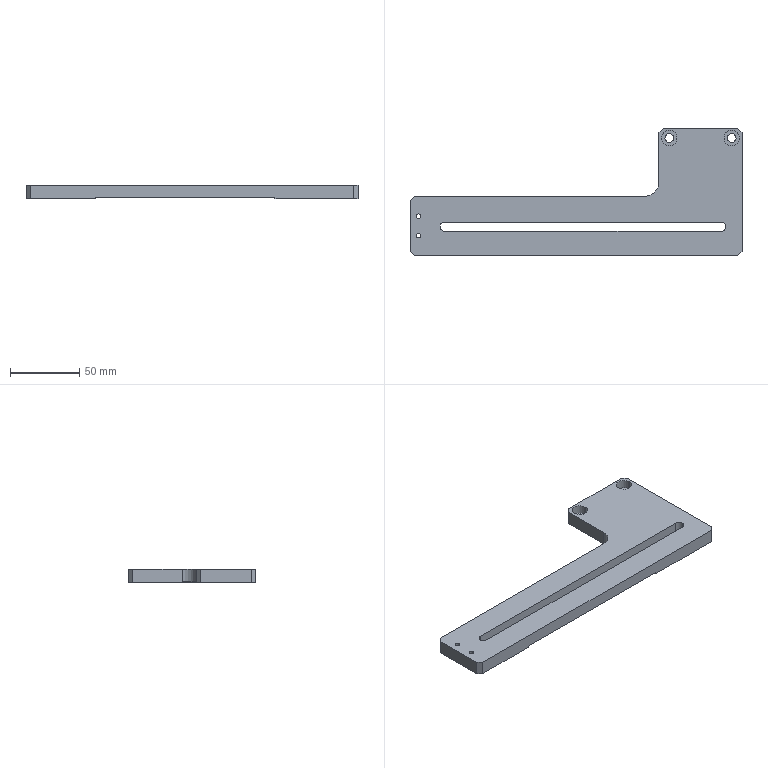Part | SolidWorks | features ICE 3, HoleWzd 2, Chamfer 1, Extrusion 1, Fillet 1 | 1 solid | 39 faces | box 240 x 92 x 10 mm | volume 112675 mm3 | plane 23 | cylinder 16 | commonest cylinder face diameters 3.3 x4 6.4 x4 11 x4 6.6 x3 20 x1
STEP:
#1=CARTESIAN_POINT('',(62.,39.,3.6));
#2=VERTEX_POINT('',#1);
#3=CARTESIAN_POINT('',(73.,39.,3.6));
#4=VERTEX_POINT('',#3);
#5=CARTESIAN_POINT('',(67.5,39.,3.6));
#6=DIRECTION('',(0.,0.,1.));
#7=DIRECTION('',(1.,0.,0.));
#8=AXIS2_PLACEMENT_3D('',#5,#6,#7);
#9=CIRCLE('',#8,5.5);
#10=EDGE_CURVE('',#2,#4,#9,.T.);
#11=ORIENTED_EDGE('',*,*,#10,.F.);
#12=CARTESIAN_POINT('',(62.,39.,10.));
#13=VERTEX_POINT('',#12);
#14=CARTESIAN_POINT('',(62.,39.,10.));
#15=DIRECTION('',(0.,0.,1.));
#16=VECTOR('',#15,1000.);
#17=LINE('',#14,#16);
#18=EDGE_CURVE('',#2,#13,#17,.T.);
#19=ORIENTED_EDGE('',*,*,#18,.T.);
#20=CARTESIAN_POINT('',(73.,39.,10.));
#21=VERTEX_POINT('',#20);
#22=CARTESIAN_POINT('',(67.5,39.,10.));
#23=DIRECTION('',(0.,0.,1.));
#24=DIRECTION('',(1.,0.,0.));
#25=AXIS2_PLACEMENT_3D('',#22,#23,#24);
#26=CIRCLE('',#25,5.5);
#27=EDGE_CURVE('',#13,#21,#26,.T.);
#28=ORIENTED_EDGE('',*,*,#27,.T.);
#29=CARTESIAN_POINT('',(73.,39.,10.));
#30=DIRECTION('',(0.,0.,1.));
#31=VECTOR('',#30,1000.);
#32=LINE('',#29,#31);
#33=EDGE_CURVE('',#4,#21,#32,.T.);
#34=ORIENTED_EDGE('',*,*,#33,.F.);
#35=EDGE_LOOP('',(#11,#19,#28,#34));
#36=FACE_OUTER_BOUND('',#35,.T.);
#37=CARTESIAN_POINT('',(67.5,39.,10.));
#38=DIRECTION('',(0.,0.,1.));
#39=DIRECTION('',(1.,0.,0.));
#40=AXIS2_PLACEMENT_3D('',#37,#38,#39);
#41=CYLINDRICAL_SURFACE('',#40,5.5);
#42=ADVANCED_FACE('',(#36),#41,.F.);
#43=CARTESIAN_POINT('',(64.3,39.,0.));
#44=VERTEX_POINT('',#43);
#45=CARTESIAN_POINT('',(70.7,39.,0.));
#46=VERTEX_POINT('',#45);
#47=CARTESIAN_POINT('',(67.5,39.,0.));
#48=DIRECTION('',(0.,0.,1.));
#49=DIRECTION('',(1.,0.,0.));
#50=AXIS2_PLACEMENT_3D('',#47,#48,#49);
#51=CIRCLE('',#50,3.2);
#52=EDGE_CURVE('',#44,#46,#51,.T.);
#53=ORIENTED_EDGE('',*,*,#52,.F.);
#54=CARTESIAN_POINT('',(64.3,39.,3.6));
#55=VERTEX_POINT('',#54);
#56=CARTESIAN_POINT('',(64.3,39.,10.));
#57=DIRECTION('',(0.,0.,1.));
#58=VECTOR('',#57,1000.);
#59=LINE('',#56,#58);
#60=EDGE_CURVE('',#44,#55,#59,.T.);
#61=ORIENTED_EDGE('',*,*,#60,.T.);
#62=CARTESIAN_POINT('',(70.7,39.,3.6));
#63=VERTEX_POINT('',#62);
#64=CARTESIAN_POINT('',(67.5,39.,3.6));
#65=DIRECTION('',(0.,0.,1.));
#66=DIRECTION('',(1.,0.,0.));
#67=AXIS2_PLACEMENT_3D('',#64,#65,#66);
#68=CIRCLE('',#67,3.2);
#69=EDGE_CURVE('',#55,#63,#68,.T.);
#70=ORIENTED_EDGE('',*,*,#69,.T.);
#71=CARTESIAN_POINT('',(70.7,39.,10.));
#72=DIRECTION('',(0.,0.,1.));
#73=VECTOR('',#72,1000.);
#74=LINE('',#71,#73);
#75=EDGE_CURVE('',#46,#63,#74,.T.);
#76=ORIENTED_EDGE('',*,*,#75,.F.);
#77=EDGE_LOOP('',(#53,#61,#70,#76));
#78=FACE_OUTER_BOUND('',#77,.T.);
#79=CARTESIAN_POINT('',(67.5,39.,10.));
#80=DIRECTION('',(0.,0.,1.));
#81=DIRECTION('',(1.,0.,0.));
#82=AXIS2_PLACEMENT_3D('',#79,#80,#81);
#83=CYLINDRICAL_SURFACE('',#82,3.2);
#84=ADVANCED_FACE('',(#78),#83,.F.);
#85=CARTESIAN_POINT('',(107.,39.,3.6));
#86=VERTEX_POINT('',#85);
#87=CARTESIAN_POINT('',(118.,39.,3.6));
#88=VERTEX_POINT('',#87);
#89=CARTESIAN_POINT('',(112.5,39.,3.6));
#90=DIRECTION('',(0.,0.,1.));
#91=DIRECTION('',(1.,0.,0.));
#92=AXIS2_PLACEMENT_3D('',#89,#90,#91);
#93=CIRCLE('',#92,5.5);
#94=EDGE_CURVE('',#86,#88,#93,.T.);
#95=ORIENTED_EDGE('',*,*,#94,.F.);
#96=CARTESIAN_POINT('',(107.,39.,10.));
#97=VERTEX_POINT('',#96);
#98=CARTESIAN_POINT('',(107.,39.,10.));
#99=DIRECTION('',(0.,0.,1.));
#100=VECTOR('',#99,1000.);
#101=LINE('',#98,#100);
#102=EDGE_CURVE('',#86,#97,#101,.T.);
#103=ORIENTED_EDGE('',*,*,#102,.T.);
#104=CARTESIAN_POINT('',(118.,39.,10.));
#105=VERTEX_POINT('',#104);
#106=CARTESIAN_POINT('',(112.5,39.,10.));
#107=DIRECTION('',(0.,0.,1.));
#108=DIRECTION('',(1.,0.,0.));
#109=AXIS2_PLACEMENT_3D('',#106,#107,#108);
#110=CIRCLE('',#109,5.5);
#111=EDGE_CURVE('',#97,#105,#110,.T.);
#112=ORIENTED_EDGE('',*,*,#111,.T.);
#113=CARTESIAN_POINT('',(118.,39.,10.));
#114=DIRECTION('',(0.,0.,1.));
#115=VECTOR('',#114,1000.);
#116=LINE('',#113,#115);
#117=EDGE_CURVE('',#88,#105,#116,.T.);
#118=ORIENTED_EDGE('',*,*,#117,.F.);
#119=EDGE_LOOP('',(#95,#103,#112,#118));
#120=FACE_OUTER_BOUND('',#119,.T.);
#121=CARTESIAN_POINT('',(112.5,39.,10.));
#122=DIRECTION('',(0.,0.,1.));
#123=DIRECTION('',(1.,0.,0.));
#124=AXIS2_PLACEMENT_3D('',#121,#122,#123);
#125=CYLINDRICAL_SURFACE('',#124,5.5);
#126=ADVANCED_FACE('',(#120),#125,.F.);
#127=CARTESIAN_POINT('',(109.3,39.,0.));
#128=VERTEX_POINT('',#127);
#129=CARTESIAN_POINT('',(115.7,39.,0.));
#130=VERTEX_POINT('',#129);
#131=CARTESIAN_POINT('',(112.5,39.,0.));
#132=DIRECTION('',(0.,0.,1.));
#133=DIRECTION('',(1.,0.,0.));
#134=AXIS2_PLACEMENT_3D('',#131,#132,#133);
#135=CIRCLE('',#134,3.2);
#136=EDGE_CURVE('',#128,#130,#135,.T.);
#137=ORIENTED_EDGE('',*,*,#136,.F.);
#138=CARTESIAN_POINT('',(109.3,39.,3.6));
#139=VERTEX_POINT('',#138);
#140=CARTESIAN_POINT('',(109.3,39.,10.));
#141=DIRECTION('',(0.,0.,1.));
#142=VECTOR('',#141,1000.);
#143=LINE('',#140,#142);
#144=EDGE_CURVE('',#128,#139,#143,.T.);
#145=ORIENTED_EDGE('',*,*,#144,.T.);
#146=CARTESIAN_POINT('',(115.7,39.,3.6));
#147=VERTEX_POINT('',#146);
#148=CARTESIAN_POINT('',(112.5,39.,3.6));
#149=DIRECTION('',(0.,0.,1.));
#150=DIRECTION('',(1.,0.,0.));
#151=AXIS2_PLACEMENT_3D('',#148,#149,#150);
#152=CIRCLE('',#151,3.2);
#153=EDGE_CURVE('',#139,#147,#152,.T.);
#154=ORIENTED_EDGE('',*,*,#153,.T.);
#155=CARTESIAN_POINT('',(115.7,39.,10.));
#156=DIRECTION('',(0.,0.,1.));
#157=VECTOR('',#156,1000.);
#158=LINE('',#155,#157);
#159=EDGE_CURVE('',#130,#147,#158,.T.);
#160=ORIENTED_EDGE('',*,*,#159,.F.);
#161=EDGE_LOOP('',(#137,#145,#154,#160));
#162=FACE_OUTER_BOUND('',#161,.T.);
#163=CARTESIAN_POINT('',(112.5,39.,10.));
#164=DIRECTION('',(0.,0.,1.));
#165=DIRECTION('',(1.,0.,0.));
#166=AXIS2_PLACEMENT_3D('',#163,#164,#165);
#167=CYLINDRICAL_SURFACE('',#166,3.2);
#168=ADVANCED_FACE('',(#162),#167,.F.);
#169=CARTESIAN_POINT('',(-115.65,-17.5,0.));
#170=VERTEX_POINT('',#169);
#171=CARTESIAN_POINT('',(-112.35,-17.5,0.));
#172=VERTEX_POINT('',#171);
#173=CARTESIAN_POINT('',(-114.,-17.5,0.));
#174=DIRECTION('',(0.,0.,1.));
#175=DIRECTION('',(1.,0.,0.));
#176=AXIS2_PLACEMENT_3D('',#173,#174,#175);
#177=CIRCLE('',#176,1.65);
#178=EDGE_CURVE('',#170,#172,#177,.T.);
#179=ORIENTED_EDGE('',*,*,#178,.F.);
#180=CARTESIAN_POINT('',(-115.65,-17.5,10.));
#181=VERTEX_POINT('',#180);
#182=CARTESIAN_POINT('',(-115.65,-17.5,10.));
#183=DIRECTION('',(0.,0.,1.));
#184=VECTOR('',#183,1000.);
#185=LINE('',#182,#184);
#186=EDGE_CURVE('',#170,#181,#185,.T.);
#187=ORIENTED_EDGE('',*,*,#186,.T.);
#188=CARTESIAN_POINT('',(-112.35,-17.5,10.));
#189=VERTEX_POINT('',#188);
#190=CARTESIAN_POINT('',(-114.,-17.5,10.));
#191=DIRECTION('',(0.,0.,1.));
#192=DIRECTION('',(1.,0.,0.));
#193=AXIS2_PLACEMENT_3D('',#190,#191,#192);
#194=CIRCLE('',#193,1.65);
#195=EDGE_CURVE('',#181,#189,#194,.T.);
#196=ORIENTED_EDGE('',*,*,#195,.T.);
#197=CARTESIAN_POINT('',(-112.35,-17.5,10.));
#198=DIRECTION('',(0.,0.,1.));
#199=VECTOR('',#198,1000.);
#200=LINE('',#197,#199);
#201=EDGE_CURVE('',#172,#189,#200,.T.);
#202=ORIENTED_EDGE('',*,*,#201,.F.);
#203=EDGE_LOOP('',(#179,#187,#196,#202));
#204=FACE_OUTER_BOUND('',#203,.T.);
#205=CARTESIAN_POINT('',(-114.,-17.5,10.));
#206=DIRECTION('',(0.,0.,1.));
#207=DIRECTION('',(1.,0.,0.));
#208=AXIS2_PLACEMENT_3D('',#205,#206,#207);
#209=CYLINDRICAL_SURFACE('',#208,1.65);
#210=ADVANCED_FACE('',(#204),#209,.F.);
#211=CARTESIAN_POINT('',(-115.65,-31.5,0.));
#212=VERTEX_POINT('',#211);
#213=CARTESIAN_POINT('',(-112.35,-31.5,0.));
#214=VERTEX_POINT('',#213);
#215=CARTESIAN_POINT('',(-114.,-31.5,0.));
#216=DIRECTION('',(0.,0.,1.));
#217=DIRECTION('',(1.,0.,0.));
#218=AXIS2_PLACEMENT_3D('',#215,#216,#217);
#219=CIRCLE('',#218,1.65);
#220=EDGE_CURVE('',#212,#214,#219,.T.);
#221=ORIENTED_EDGE('',*,*,#220,.F.);
#222=CARTESIAN_POINT('',(-115.65,-31.5,10.));
#223=VERTEX_POINT('',#222);
#224=CARTESIAN_POINT('',(-115.65,-31.5,10.));
#225=DIRECTION('',(0.,0.,1.));
#226=VECTOR('',#225,1000.);
#227=LINE('',#224,#226);
#228=EDGE_CURVE('',#212,#223,#227,.T.);
#229=ORIENTED_EDGE('',*,*,#228,.T.);
#230=CARTESIAN_POINT('',(-112.35,-31.5,10.));
#231=VERTEX_POINT('',#230);
#232=CARTESIAN_POINT('',(-114.,-31.5,10.));
#233=DIRECTION('',(0.,0.,1.));
#234=DIRECTION('',(1.,0.,0.));
#235=AXIS2_PLACEMENT_3D('',#232,#233,#234);
#236=CIRCLE('',#235,1.65);
#237=EDGE_CURVE('',#223,#231,#236,.T.);
#238=ORIENTED_EDGE('',*,*,#237,.T.);
#239=CARTESIAN_POINT('',(-112.35,-31.5,10.));
#240=DIRECTION('',(0.,0.,1.));
#241=VECTOR('',#240,1000.);
#242=LINE('',#239,#241);
#243=EDGE_CURVE('',#214,#231,#242,.T.);
#244=ORIENTED_EDGE('',*,*,#243,.F.);
#245=EDGE_LOOP('',(#221,#229,#238,#244));
#246=FACE_OUTER_BOUND('',#245,.T.);
#247=CARTESIAN_POINT('',(-114.,-31.5,10.));
#248=DIRECTION('',(0.,0.,1.));
#249=DIRECTION('',(1.,0.,0.));
#250=AXIS2_PLACEMENT_3D('',#247,#248,#249);
#251=CYLINDRICAL_SURFACE('',#250,1.65);
#252=ADVANCED_FACE('',(#246),#251,.F.);
#253=CARTESIAN_POINT('',(108.3,-25.,0.));
#254=VERTEX_POINT('',#253);
#255=CARTESIAN_POINT('',(105.,-21.7,0.));
#256=VERTEX_POINT('',#255);
#257=CARTESIAN_POINT('',(105.,-25.,0.));
#258=DIRECTION('',(0.,0.,1.));
#259=DIRECTION('',(1.,0.,0.));
#260=AXIS2_PLACEMENT_3D('',#257,#258,#259);
#261=CIRCLE('',#260,3.3);
#262=EDGE_CURVE('',#254,#256,#261,.T.);
#263=ORIENTED_EDGE('',*,*,#262,.F.);
#264=CARTESIAN_POINT('',(108.3,-25.,10.));
#265=VERTEX_POINT('',#264);
#266=CARTESIAN_POINT('',(108.3,-25.,0.));
#267=DIRECTION('',(0.,0.,1.));
#268=VECTOR('',#267,1000.);
#269=LINE('',#266,#268);
#270=EDGE_CURVE('',#254,#265,#269,.T.);
#271=ORIENTED_EDGE('',*,*,#270,.T.);
#272=CARTESIAN_POINT('',(105.,-21.7,10.));
#273=VERTEX_POINT('',#272);
#274=CARTESIAN_POINT('',(105.,-25.,10.));
#275=DIRECTION('',(0.,0.,1.));
#276=DIRECTION('',(1.,0.,0.));
#277=AXIS2_PLACEMENT_3D('',#274,#275,#276);
#278=CIRCLE('',#277,3.3);
#279=EDGE_CURVE('',#265,#273,#278,.T.);
#280=ORIENTED_EDGE('',*,*,#279,.T.);
#281=CARTESIAN_POINT('',(105.,-21.7,0.));
#282=DIRECTION('',(0.,0.,1.));
#283=VECTOR('',#282,1000.);
#284=LINE('',#281,#283);
#285=EDGE_CURVE('',#256,#273,#284,.T.);
#286=ORIENTED_EDGE('',*,*,#285,.F.);
#287=EDGE_LOOP('',(#263,#271,#280,#286));
#288=FACE_OUTER_BOUND('',#287,.T.);
#289=CARTESIAN_POINT('',(105.,-25.,0.));
#290=DIRECTION('',(0.,0.,1.));
#291=DIRECTION('',(1.,0.,0.));
#292=AXIS2_PLACEMENT_3D('',#289,#290,#291);
#293=CYLINDRICAL_SURFACE('',#292,3.3);
#294=ADVANCED_FACE('',(#288),#293,.F.);
#295=CARTESIAN_POINT('',(-114.,-31.5,0.));
#296=DIRECTION('',(0.,0.,1.));
#297=DIRECTION('',(1.,0.,0.));
#298=AXIS2_PLACEMENT_3D('',#295,#296,#297);
#299=CIRCLE('',#298,1.65);
#300=EDGE_CURVE('',#214,#212,#299,.T.);
#301=ORIENTED_EDGE('',*,*,#300,.T.);
#302=ORIENTED_EDGE('',*,*,#220,.T.);
#303=EDGE_LOOP('',(#301,#302));
#304=FACE_BOUND('',#303,.T.);
#305=CARTESIAN_POINT('',(-114.,-17.5,0.));
#306=DIRECTION('',(0.,0.,1.));
#307=DIRECTION('',(1.,0.,0.));
#308=AXIS2_PLACEMENT_3D('',#305,#306,#307);
#309=CIRCLE('',#308,1.65);
#310=EDGE_CURVE('',#172,#170,#309,.T.);
#311=ORIENTED_EDGE('',*,*,#310,.T.);
#312=ORIENTED_EDGE('',*,*,#178,.T.);
#313=EDGE_LOOP('',(#311,#312));
#314=FACE_BOUND('',#313,.T.);
#315=CARTESIAN_POINT('',(-117.,-3.,0.));
#316=VERTEX_POINT('',#315);
#317=CARTESIAN_POINT('',(-70.,-3.,0.));
#318=VERTEX_POINT('',#317);
#319=CARTESIAN_POINT('',(-120.,-3.,0.));
#320=DIRECTION('',(1.,0.,0.));
#321=VECTOR('',#320,1000.);
#322=LINE('',#319,#321);
#323=EDGE_CURVE('',#316,#318,#322,.T.);
#324=ORIENTED_EDGE('',*,*,#323,.T.);
#325=CARTESIAN_POINT('',(-70.,-21.7,0.));
#326=VERTEX_POINT('',#325);
#327=CARTESIAN_POINT('',(-70.,-46.,0.));
#328=DIRECTION('',(0.,1.,0.));
#329=VECTOR('',#328,1000.);
#330=LINE('',#327,#329);
#331=EDGE_CURVE('',#326,#318,#330,.T.);
#332=ORIENTED_EDGE('',*,*,#331,.F.);
#333=CARTESIAN_POINT('',(-95.,-21.7,0.));
#334=VERTEX_POINT('',#333);
#335=CARTESIAN_POINT('',(-95.,-21.7,0.));
#336=DIRECTION('',(-1.,0.,0.));
#337=VECTOR('',#336,1000.);
#338=LINE('',#335,#337);
#339=EDGE_CURVE('',#326,#334,#338,.T.);
#340=ORIENTED_EDGE('',*,*,#339,.T.);
#341=CARTESIAN_POINT('',(-95.,-28.3,0.));
#342=VERTEX_POINT('',#341);
#343=CARTESIAN_POINT('',(-95.,-25.,0.));
#344=DIRECTION('',(0.,0.,1.));
#345=DIRECTION('',(1.,0.,0.));
#346=AXIS2_PLACEMENT_3D('',#343,#344,#345);
#347=CIRCLE('',#346,3.3);
#348=EDGE_CURVE('',#334,#342,#347,.T.);
#349=ORIENTED_EDGE('',*,*,#348,.T.);
#350=CARTESIAN_POINT('',(-70.,-28.3,0.));
#351=VERTEX_POINT('',#350);
#352=CARTESIAN_POINT('',(-95.,-28.3,0.));
#353=DIRECTION('',(1.,0.,0.));
#354=VECTOR('',#353,1000.);
#355=LINE('',#352,#354);
#356=EDGE_CURVE('',#342,#351,#355,.T.);
#357=ORIENTED_EDGE('',*,*,#356,.T.);
#358=CARTESIAN_POINT('',(-70.,-46.,0.));
#359=VERTEX_POINT('',#358);
#360=CARTESIAN_POINT('',(-70.,-46.,0.));
#361=DIRECTION('',(0.,1.,0.));
#362=VECTOR('',#361,1000.);
#363=LINE('',#360,#362);
#364=EDGE_CURVE('',#359,#351,#363,.T.);
#365=ORIENTED_EDGE('',*,*,#364,.F.);
#366=CARTESIAN_POINT('',(-117.,-46.,0.));
#367=VERTEX_POINT('',#366);
#368=CARTESIAN_POINT('',(-120.,-46.,0.));
#369=DIRECTION('',(1.,0.,0.));
#370=VECTOR('',#369,1000.);
#371=LINE('',#368,#370);
#372=EDGE_CURVE('',#367,#359,#371,.T.);
#373=ORIENTED_EDGE('',*,*,#372,.F.);
#374=CARTESIAN_POINT('',(-120.,-43.,0.));
#375=VERTEX_POINT('',#374);
#376=CARTESIAN_POINT('',(-117.,-46.,0.));
#377=DIRECTION('',(-0.7071,0.7071,0.));
#378=VECTOR('',#377,1000.);
#379=LINE('',#376,#378);
#380=EDGE_CURVE('',#367,#375,#379,.T.);
#381=ORIENTED_EDGE('',*,*,#380,.T.);
#382=CARTESIAN_POINT('',(-120.,-6.,0.));
#383=VERTEX_POINT('',#382);
#384=CARTESIAN_POINT('',(-120.,46.,0.));
#385=DIRECTION('',(0.,-1.,0.));
#386=VECTOR('',#385,1000.);
#387=LINE('',#384,#386);
#388=EDGE_CURVE('',#383,#375,#387,.T.);
#389=ORIENTED_EDGE('',*,*,#388,.F.);
#390=CARTESIAN_POINT('',(-117.,-3.,0.));
#391=DIRECTION('',(0.7071,0.7071,0.));
#392=VECTOR('',#391,1000.);
#393=LINE('',#390,#392);
#394=EDGE_CURVE('',#383,#316,#393,.T.);
#395=ORIENTED_EDGE('',*,*,#394,.T.);
#396=EDGE_LOOP('',(#324,#332,#340,#349,#357,#365,#373,#381,#389,#395));
#397=FACE_OUTER_BOUND('',#396,.T.);
#398=CARTESIAN_POINT('',(0.,0.,0.));
#399=DIRECTION('',(0.,0.,1.));
#400=DIRECTION('',(1.,0.,0.));
#401=AXIS2_PLACEMENT_3D('',#398,#399,#400);
#402=PLANE('',#401);
#403=ADVANCED_FACE('',(#304,#314,#397),#402,.F.);
#404=CARTESIAN_POINT('',(50.,-3.,1.));
#405=VERTEX_POINT('',#404);
#406=CARTESIAN_POINT('',(60.,7.,1.));
#407=VERTEX_POINT('',#406);
#408=CARTESIAN_POINT('',(50.,7.,1.));
#409=DIRECTION('',(0.,0.,1.));
#410=DIRECTION('',(-1.,0.,0.));
#411=AXIS2_PLACEMENT_3D('',#408,#409,#410);
#412=CIRCLE('',#411,10.);
#413=EDGE_CURVE('',#405,#407,#412,.T.);
#414=ORIENTED_EDGE('',*,*,#413,.F.);
#415=CARTESIAN_POINT('',(50.,-3.,10.));
#416=VERTEX_POINT('',#415);
#417=CARTESIAN_POINT('',(50.,-3.,0.));
#418=DIRECTION('',(0.,0.,-1.));
#419=VECTOR('',#418,1000.);
#420=LINE('',#417,#419);
#421=EDGE_CURVE('',#416,#405,#420,.T.);
#422=ORIENTED_EDGE('',*,*,#421,.F.);
#423=CARTESIAN_POINT('',(60.,7.,10.));
#424=VERTEX_POINT('',#423);
#425=CARTESIAN_POINT('',(50.,7.,10.));
#426=DIRECTION('',(0.,0.,-1.));
#427=DIRECTION('',(1.,0.,0.));
#428=AXIS2_PLACEMENT_3D('',#425,#426,#427);
#429=CIRCLE('',#428,10.);
#430=EDGE_CURVE('',#424,#416,#429,.T.);
#431=ORIENTED_EDGE('',*,*,#430,.F.);
#432=CARTESIAN_POINT('',(60.,7.,10.));
#433=DIRECTION('',(0.,0.,1.));
#434=VECTOR('',#433,1000.);
#435=LINE('',#432,#434);
#436=EDGE_CURVE('',#407,#424,#435,.T.);
#437=ORIENTED_EDGE('',*,*,#436,.F.);
#438=EDGE_LOOP('',(#414,#422,#431,#437));
#439=FACE_OUTER_BOUND('',#438,.T.);
#440=CARTESIAN_POINT('',(50.,7.,0.));
#441=DIRECTION('',(0.,0.,-1.));
#442=DIRECTION('',(-1.,0.,0.));
#443=AXIS2_PLACEMENT_3D('',#440,#441,#442);
#444=CYLINDRICAL_SURFACE('',#443,10.);
#445=ADVANCED_FACE('',(#439),#444,.F.);
#446=CARTESIAN_POINT('',(120.,-43.,10.));
#447=VERTEX_POINT('',#446);
#448=CARTESIAN_POINT('',(120.,43.,10.));
#449=VERTEX_POINT('',#448);
#450=CARTESIAN_POINT('',(120.,46.,10.));
#451=DIRECTION('',(0.,1.,0.));
#452=VECTOR('',#451,1000.);
#453=LINE('',#450,#452);
#454=EDGE_CURVE('',#447,#449,#453,.T.);
#455=ORIENTED_EDGE('',*,*,#454,.F.);
#456=CARTESIAN_POINT('',(120.,-43.,0.));
#457=VERTEX_POINT('',#456);
#458=CARTESIAN_POINT('',(120.,-43.,10.));
#459=DIRECTION('',(0.,0.,-1.));
#460=VECTOR('',#459,1000.);
#461=LINE('',#458,#460);
#462=EDGE_CURVE('',#447,#457,#461,.T.);
#463=ORIENTED_EDGE('',*,*,#462,.T.);
#464=CARTESIAN_POINT('',(120.,43.,0.));
#465=VERTEX_POINT('',#464);
#466=CARTESIAN_POINT('',(120.,46.,0.));
#467=DIRECTION('',(0.,1.,0.));
#468=VECTOR('',#467,1000.);
#469=LINE('',#466,#468);
#470=EDGE_CURVE('',#457,#465,#469,.T.);
#471=ORIENTED_EDGE('',*,*,#470,.T.);
#472=CARTESIAN_POINT('',(120.,43.,10.));
#473=DIRECTION('',(0.,0.,1.));
#474=VECTOR('',#473,1000.);
#475=LINE('',#472,#474);
#476=EDGE_CURVE('',#465,#449,#475,.T.);
#477=ORIENTED_EDGE('',*,*,#476,.T.);
#478=EDGE_LOOP('',(#455,#463,#471,#477));
#479=FACE_OUTER_BOUND('',#478,.T.);
#480=CARTESIAN_POINT('',(120.,46.,10.));
#481=DIRECTION('',(-1.,0.,0.));
#482=DIRECTION('',(0.,0.,1.));
#483=AXIS2_PLACEMENT_3D('',#480,#481,#482);
#484=PLANE('',#483);
#485=ADVANCED_FACE('',(#479),#484,.F.);
#486=CARTESIAN_POINT('',(117.,46.,10.));
#487=VERTEX_POINT('',#486);
#488=CARTESIAN_POINT('',(63.,46.,10.));
#489=VERTEX_POINT('',#488);
#490=CARTESIAN_POINT('',(-120.,46.,10.));
#491=DIRECTION('',(-1.,0.,0.));
#492=VECTOR('',#491,1000.);
#493=LINE('',#490,#492);
#494=EDGE_CURVE('',#487,#489,#493,.T.);
#495=ORIENTED_EDGE('',*,*,#494,.F.);
#496=CARTESIAN_POINT('',(117.,46.,0.));
#497=VERTEX_POINT('',#496);
#498=CARTESIAN_POINT('',(117.,46.,10.));
#499=DIRECTION('',(0.,0.,-1.));
#500=VECTOR('',#499,1000.);
#501=LINE('',#498,#500);
#502=EDGE_CURVE('',#487,#497,#501,.T.);
#503=ORIENTED_EDGE('',*,*,#502,.T.);
#504=CARTESIAN_POINT('',(63.,46.,0.));
#505=VERTEX_POINT('',#504);
#506=CARTESIAN_POINT('',(-120.,46.,0.));
#507=DIRECTION('',(-1.,0.,0.));
#508=VECTOR('',#507,1000.);
#509=LINE('',#506,#508);
#510=EDGE_CURVE('',#497,#505,#509,.T.);
#511=ORIENTED_EDGE('',*,*,#510,.T.);
#512=CARTESIAN_POINT('',(63.,46.,10.));
#513=DIRECTION('',(0.,0.,1.));
#514=VECTOR('',#513,1000.);
#515=LINE('',#512,#514);
#516=EDGE_CURVE('',#505,#489,#515,.T.);
#517=ORIENTED_EDGE('',*,*,#516,.T.);
#518=EDGE_LOOP('',(#495,#503,#511,#517));
#519=FACE_OUTER_BOUND('',#518,.T.);
#520=CARTESIAN_POINT('',(-120.,46.,10.));
#521=DIRECTION('',(0.,-1.,0.));
#522=DIRECTION('',(0.,0.,-1.));
#523=AXIS2_PLACEMENT_3D('',#520,#521,#522);
#524=PLANE('',#523);
#525=ADVANCED_FACE('',(#519),#524,.F.);
#526=ORIENTED_EDGE('',*,*,#388,.T.);
#527=CARTESIAN_POINT('',(-120.,-43.,10.));
#528=VERTEX_POINT('',#527);
#529=CARTESIAN_POINT('',(-120.,-43.,10.));
#530=DIRECTION('',(0.,0.,1.));
#531=VECTOR('',#530,1000.);
#532=LINE('',#529,#531);
#533=EDGE_CURVE('',#375,#528,#532,.T.);
#534=ORIENTED_EDGE('',*,*,#533,.T.);
#535=CARTESIAN_POINT('',(-120.,-6.,10.));
#536=VERTEX_POINT('',#535);
#537=CARTESIAN_POINT('',(-120.,46.,10.));
#538=DIRECTION('',(0.,-1.,0.));
#539=VECTOR('',#538,1000.);
#540=LINE('',#537,#539);
#541=EDGE_CURVE('',#536,#528,#540,.T.);
#542=ORIENTED_EDGE('',*,*,#541,.F.);
#543=CARTESIAN_POINT('',(-120.,-6.,10.));
#544=DIRECTION('',(0.,0.,-1.));
#545=VECTOR('',#544,1000.);
#546=LINE('',#543,#545);
#547=EDGE_CURVE('',#536,#383,#546,.T.);
#548=ORIENTED_EDGE('',*,*,#547,.T.);
#549=EDGE_LOOP('',(#526,#534,#542,#548));
#550=FACE_OUTER_BOUND('',#549,.T.);
#551=CARTESIAN_POINT('',(-120.,46.,10.));
#552=DIRECTION('',(1.,0.,0.));
#553=DIRECTION('',(0.,0.,-1.));
#554=AXIS2_PLACEMENT_3D('',#551,#552,#553);
#555=PLANE('',#554);
#556=ADVANCED_FACE('',(#550),#555,.F.);
#557=ORIENTED_EDGE('',*,*,#372,.T.);
#558=CARTESIAN_POINT('',(-70.,-46.,1.));
#559=VERTEX_POINT('',#558);
#560=CARTESIAN_POINT('',(-70.,-46.,1.));
#561=DIRECTION('',(0.,0.,-1.));
#562=VECTOR('',#561,1000.);
#563=LINE('',#560,#562);
#564=EDGE_CURVE('',#559,#359,#563,.T.);
#565=ORIENTED_EDGE('',*,*,#564,.F.);
#566=CARTESIAN_POINT('',(60.,-46.,1.));
#567=VERTEX_POINT('',#566);
#568=CARTESIAN_POINT('',(-70.,-46.,1.));
#569=DIRECTION('',(-1.,0.,0.));
#570=VECTOR('',#569,1000.);
#571=LINE('',#568,#570);
#572=EDGE_CURVE('',#567,#559,#571,.T.);
#573=ORIENTED_EDGE('',*,*,#572,.F.);
#574=CARTESIAN_POINT('',(60.,-46.,0.));
#575=VERTEX_POINT('',#574);
#576=CARTESIAN_POINT('',(60.,-46.,1.));
#577=DIRECTION('',(0.,0.,-1.));
#578=VECTOR('',#577,1000.);
#579=LINE('',#576,#578);
#580=EDGE_CURVE('',#567,#575,#579,.T.);
#581=ORIENTED_EDGE('',*,*,#580,.T.);
#582=CARTESIAN_POINT('',(117.,-46.,0.));
#583=VERTEX_POINT('',#582);
#584=CARTESIAN_POINT('',(-120.,-46.,0.));
#585=DIRECTION('',(1.,0.,0.));
#586=VECTOR('',#585,1000.);
#587=LINE('',#584,#586);
#588=EDGE_CURVE('',#575,#583,#587,.T.);
#589=ORIENTED_EDGE('',*,*,#588,.T.);
#590=CARTESIAN_POINT('',(117.,-46.,10.));
#591=VERTEX_POINT('',#590);
#592=CARTESIAN_POINT('',(117.,-46.,10.));
#593=DIRECTION('',(0.,0.,1.));
#594=VECTOR('',#593,1000.);
#595=LINE('',#592,#594);
#596=EDGE_CURVE('',#583,#591,#595,.T.);
#597=ORIENTED_EDGE('',*,*,#596,.T.);
#598=CARTESIAN_POINT('',(-117.,-46.,10.));
#599=VERTEX_POINT('',#598);
#600=CARTESIAN_POINT('',(-120.,-46.,10.));
#601=DIRECTION('',(1.,0.,0.));
#602=VECTOR('',#601,1000.);
#603=LINE('',#600,#602);
#604=EDGE_CURVE('',#599,#591,#603,.T.);
#605=ORIENTED_EDGE('',*,*,#604,.F.);
#606=CARTESIAN_POINT('',(-117.,-46.,10.));
#607=DIRECTION('',(0.,0.,-1.));
#608=VECTOR('',#607,1000.);
#609=LINE('',#606,#608);
#610=EDGE_CURVE('',#599,#367,#609,.T.);
#611=ORIENTED_EDGE('',*,*,#610,.T.);
#612=EDGE_LOOP('',(#557,#565,#573,#581,#589,#597,#605,#611));
#613=FACE_OUTER_BOUND('',#612,.T.);
#614=CARTESIAN_POINT('',(-120.,-46.,10.));
#615=DIRECTION('',(0.,1.,0.));
#616=DIRECTION('',(0.,0.,1.));
#617=AXIS2_PLACEMENT_3D('',#614,#615,#616);
#618=PLANE('',#617);
#619=ADVANCED_FACE('',(#613),#618,.F.);
#620=CARTESIAN_POINT('',(67.5,39.,10.));
#621=DIRECTION('',(0.,0.,1.));
#622=DIRECTION('',(1.,0.,0.));
#623=AXIS2_PLACEMENT_3D('',#620,#621,#622);
#624=CIRCLE('',#623,5.5);
#625=EDGE_CURVE('',#21,#13,#624,.T.);
#626=ORIENTED_EDGE('',*,*,#625,.F.);
#627=ORIENTED_EDGE('',*,*,#27,.F.);
#628=EDGE_LOOP('',(#626,#627));
#629=FACE_BOUND('',#628,.T.);
#630=CARTESIAN_POINT('',(112.5,39.,10.));
#631=DIRECTION('',(0.,0.,1.));
#632=DIRECTION('',(1.,0.,0.));
#633=AXIS2_PLACEMENT_3D('',#630,#631,#632);
#634=CIRCLE('',#633,5.5);
#635=EDGE_CURVE('',#105,#97,#634,.T.);
#636=ORIENTED_EDGE('',*,*,#635,.F.);
#637=ORIENTED_EDGE('',*,*,#111,.F.);
#638=EDGE_LOOP('',(#636,#637));
#639=FACE_BOUND('',#638,.T.);
#640=CARTESIAN_POINT('',(-114.,-17.5,10.));
#641=DIRECTION('',(0.,0.,1.));
#642=DIRECTION('',(1.,0.,0.));
#643=AXIS2_PLACEMENT_3D('',#640,#641,#642);
#644=CIRCLE('',#643,1.65);
#645=EDGE_CURVE('',#189,#181,#644,.T.);
#646=ORIENTED_EDGE('',*,*,#645,.F.);
#647=ORIENTED_EDGE('',*,*,#195,.F.);
#648=EDGE_LOOP('',(#646,#647));
#649=FACE_BOUND('',#648,.T.);
#650=CARTESIAN_POINT('',(-114.,-31.5,10.));
#651=DIRECTION('',(0.,0.,1.));
#652=DIRECTION('',(1.,0.,0.));
#653=AXIS2_PLACEMENT_3D('',#650,#651,#652);
#654=CIRCLE('',#653,1.65);
#655=EDGE_CURVE('',#231,#223,#654,.T.);
#656=ORIENTED_EDGE('',*,*,#655,.F.);
#657=ORIENTED_EDGE('',*,*,#237,.F.);
#658=EDGE_LOOP('',(#656,#657));
#659=FACE_BOUND('',#658,.T.);
#660=ORIENTED_EDGE('',*,*,#541,.T.);
#661=CARTESIAN_POINT('',(-81.5,-81.5,10.));
#662=DIRECTION('',(0.7071,-0.7071,0.));
#663=VECTOR('',#662,1000.);
#664=LINE('',#661,#663);
#665=EDGE_CURVE('',#528,#599,#664,.T.);
#666=ORIENTED_EDGE('',*,*,#665,.T.);
#667=ORIENTED_EDGE('',*,*,#604,.T.);
#668=CARTESIAN_POINT('',(81.5,-81.5,10.));
#669=DIRECTION('',(0.7071,0.7071,0.));
#670=VECTOR('',#669,1000.);
#671=LINE('',#668,#670);
#672=EDGE_CURVE('',#591,#447,#671,.T.);
#673=ORIENTED_EDGE('',*,*,#672,.T.);
#674=ORIENTED_EDGE('',*,*,#454,.T.);
#675=CARTESIAN_POINT('',(81.5,81.5,10.));
#676=DIRECTION('',(-0.7071,0.7071,0.));
#677=VECTOR('',#676,1000.);
#678=LINE('',#675,#677);
#679=EDGE_CURVE('',#449,#487,#678,.T.);
#680=ORIENTED_EDGE('',*,*,#679,.T.);
#681=ORIENTED_EDGE('',*,*,#494,.T.);
#682=CARTESIAN_POINT('',(60.,43.,10.));
#683=VERTEX_POINT('',#682);
#684=CARTESIAN_POINT('',(8.5,-8.5,10.));
#685=DIRECTION('',(-0.7071,-0.7071,0.));
#686=VECTOR('',#685,1000.);
#687=LINE('',#684,#686);
#688=EDGE_CURVE('',#489,#683,#687,.T.);
#689=ORIENTED_EDGE('',*,*,#688,.T.);
#690=CARTESIAN_POINT('',(60.,46.,10.));
#691=DIRECTION('',(0.,1.,0.));
#692=VECTOR('',#691,1000.);
#693=LINE('',#690,#692);
#694=EDGE_CURVE('',#424,#683,#693,.T.);
#695=ORIENTED_EDGE('',*,*,#694,.F.);
#696=ORIENTED_EDGE('',*,*,#430,.T.);
#697=CARTESIAN_POINT('',(-117.,-3.,10.));
#698=VERTEX_POINT('',#697);
#699=CARTESIAN_POINT('',(-120.,-3.,10.));
#700=DIRECTION('',(1.,0.,0.));
#701=VECTOR('',#700,1000.);
#702=LINE('',#699,#701);
#703=EDGE_CURVE('',#698,#416,#702,.T.);
#704=ORIENTED_EDGE('',*,*,#703,.F.);
#705=CARTESIAN_POINT('',(-57.,57.,10.));
#706=DIRECTION('',(-0.7071,-0.7071,0.));
#707=VECTOR('',#706,1000.);
#708=LINE('',#705,#707);
#709=EDGE_CURVE('',#698,#536,#708,.T.);
#710=ORIENTED_EDGE('',*,*,#709,.T.);
#711=EDGE_LOOP('',(#660,#666,#667,#673,#674,#680,#681,#689,#695,#696,#704,#710));
#712=FACE_OUTER_BOUND('',#711,.T.);
#713=CARTESIAN_POINT('',(-95.,-21.7,10.));
#714=VERTEX_POINT('',#713);
#715=CARTESIAN_POINT('',(-95.,-28.3,10.));
#716=VERTEX_POINT('',#715);
#717=CARTESIAN_POINT('',(-95.,-25.,10.));
#718=DIRECTION('',(0.,0.,1.));
#719=DIRECTION('',(1.,0.,0.));
#720=AXIS2_PLACEMENT_3D('',#717,#718,#719);
#721=CIRCLE('',#720,3.3);
#722=EDGE_CURVE('',#714,#716,#721,.T.);
#723=ORIENTED_EDGE('',*,*,#722,.F.);
#724=CARTESIAN_POINT('',(-95.,-21.7,10.));
#725=DIRECTION('',(-1.,0.,0.));
#726=VECTOR('',#725,1000.);
#727=LINE('',#724,#726);
#728=EDGE_CURVE('',#273,#714,#727,.T.);
#729=ORIENTED_EDGE('',*,*,#728,.F.);
#730=ORIENTED_EDGE('',*,*,#279,.F.);
#731=CARTESIAN_POINT('',(105.,-28.3,10.));
#732=VERTEX_POINT('',#731);
#733=CARTESIAN_POINT('',(105.,-25.,10.));
#734=DIRECTION('',(0.,0.,1.));
#735=DIRECTION('',(1.,0.,0.));
#736=AXIS2_PLACEMENT_3D('',#733,#734,#735);
#737=CIRCLE('',#736,3.3);
#738=EDGE_CURVE('',#732,#265,#737,.T.);
#739=ORIENTED_EDGE('',*,*,#738,.F.);
#740=CARTESIAN_POINT('',(-95.,-28.3,10.));
#741=DIRECTION('',(1.,0.,0.));
#742=VECTOR('',#741,1000.);
#743=LINE('',#740,#742);
#744=EDGE_CURVE('',#716,#732,#743,.T.);
#745=ORIENTED_EDGE('',*,*,#744,.F.);
#746=EDGE_LOOP('',(#723,#729,#730,#739,#745));
#747=FACE_BOUND('',#746,.T.);
#748=CARTESIAN_POINT('',(0.,0.,10.));
#749=DIRECTION('',(0.,0.,1.));
#750=DIRECTION('',(1.,0.,0.));
#751=AXIS2_PLACEMENT_3D('',#748,#749,#750);
#752=PLANE('',#751);
#753=ADVANCED_FACE('',(#629,#639,#649,#659,#712,#747),#752,.T.);
#754=CARTESIAN_POINT('',(67.5,39.,0.));
#755=DIRECTION('',(0.,0.,1.));
#756=DIRECTION('',(1.,0.,0.));
#757=AXIS2_PLACEMENT_3D('',#754,#755,#756);
#758=CIRCLE('',#757,3.2);
#759=EDGE_CURVE('',#46,#44,#758,.T.);
#760=ORIENTED_EDGE('',*,*,#759,.T.);
#761=ORIENTED_EDGE('',*,*,#52,.T.);
#762=EDGE_LOOP('',(#760,#761));
#763=FACE_BOUND('',#762,.T.);
#764=CARTESIAN_POINT('',(112.5,39.,0.));
#765=DIRECTION('',(0.,0.,1.));
#766=DIRECTION('',(1.,0.,0.));
#767=AXIS2_PLACEMENT_3D('',#764,#765,#766);
#768=CIRCLE('',#767,3.2);
#769=EDGE_CURVE('',#130,#128,#768,.T.);
#770=ORIENTED_EDGE('',*,*,#769,.T.);
#771=ORIENTED_EDGE('',*,*,#136,.T.);
#772=EDGE_LOOP('',(#770,#771));
#773=FACE_BOUND('',#772,.T.);
#774=ORIENTED_EDGE('',*,*,#588,.F.);
#775=CARTESIAN_POINT('',(60.,-28.3,0.));
#776=VERTEX_POINT('',#775);
#777=CARTESIAN_POINT('',(60.,-46.,0.));
#778=DIRECTION('',(0.,-1.,0.));
#779=VECTOR('',#778,1000.);
#780=LINE('',#777,#779);
#781=EDGE_CURVE('',#776,#575,#780,.T.);
#782=ORIENTED_EDGE('',*,*,#781,.F.);
#783=CARTESIAN_POINT('',(105.,-28.3,0.));
#784=VERTEX_POINT('',#783);
#785=CARTESIAN_POINT('',(-95.,-28.3,0.));
#786=DIRECTION('',(1.,0.,0.));
#787=VECTOR('',#786,1000.);
#788=LINE('',#785,#787);
#789=EDGE_CURVE('',#776,#784,#788,.T.);
#790=ORIENTED_EDGE('',*,*,#789,.T.);
#791=CARTESIAN_POINT('',(105.,-25.,0.));
#792=DIRECTION('',(0.,0.,1.));
#793=DIRECTION('',(1.,0.,0.));
#794=AXIS2_PLACEMENT_3D('',#791,#792,#793);
#795=CIRCLE('',#794,3.3);
#796=EDGE_CURVE('',#784,#254,#795,.T.);
#797=ORIENTED_EDGE('',*,*,#796,.T.);
#798=ORIENTED_EDGE('',*,*,#262,.T.);
#799=CARTESIAN_POINT('',(60.,-21.7,0.));
#800=VERTEX_POINT('',#799);
#801=CARTESIAN_POINT('',(-95.,-21.7,0.));
#802=DIRECTION('',(-1.,0.,0.));
#803=VECTOR('',#802,1000.);
#804=LINE('',#801,#803);
#805=EDGE_CURVE('',#256,#800,#804,.T.);
#806=ORIENTED_EDGE('',*,*,#805,.T.);
#807=CARTESIAN_POINT('',(60.,43.,0.));
#808=VERTEX_POINT('',#807);
#809=CARTESIAN_POINT('',(60.,46.,0.));
#810=DIRECTION('',(0.,1.,0.));
#811=VECTOR('',#810,1000.);
#812=LINE('',#809,#811);
#813=EDGE_CURVE('',#800,#808,#812,.T.);
#814=ORIENTED_EDGE('',*,*,#813,.T.);
#815=CARTESIAN_POINT('',(63.,46.,0.));
#816=DIRECTION('',(0.7071,0.7071,0.));
#817=VECTOR('',#816,1000.);
#818=LINE('',#815,#817);
#819=EDGE_CURVE('',#808,#505,#818,.T.);
#820=ORIENTED_EDGE('',*,*,#819,.T.);
#821=ORIENTED_EDGE('',*,*,#510,.F.);
#822=CARTESIAN_POINT('',(117.,46.,0.));
#823=DIRECTION('',(0.7071,-0.7071,0.));
#824=VECTOR('',#823,1000.);
#825=LINE('',#822,#824);
#826=EDGE_CURVE('',#497,#465,#825,.T.);
#827=ORIENTED_EDGE('',*,*,#826,.T.);
#828=ORIENTED_EDGE('',*,*,#470,.F.);
#829=CARTESIAN_POINT('',(120.,-43.,0.));
#830=DIRECTION('',(-0.7071,-0.7071,0.));
#831=VECTOR('',#830,1000.);
#832=LINE('',#829,#831);
#833=EDGE_CURVE('',#457,#583,#832,.T.);
#834=ORIENTED_EDGE('',*,*,#833,.T.);
#835=EDGE_LOOP('',(#774,#782,#790,#797,#798,#806,#814,#820,#821,#827,#828,#834));
#836=FACE_OUTER_BOUND('',#835,.T.);
#837=CARTESIAN_POINT('',(0.,0.,0.));
#838=DIRECTION('',(0.,0.,1.));
#839=DIRECTION('',(1.,0.,0.));
#840=AXIS2_PLACEMENT_3D('',#837,#838,#839);
#841=PLANE('',#840);
#842=ADVANCED_FACE('',(#763,#773,#836),#841,.F.);
#843=ORIENTED_EDGE('',*,*,#722,.T.);
#844=CARTESIAN_POINT('',(-95.,-28.3,0.));
#845=DIRECTION('',(0.,0.,1.));
#846=VECTOR('',#845,1000.);
#847=LINE('',#844,#846);
#848=EDGE_CURVE('',#342,#716,#847,.T.);
#849=ORIENTED_EDGE('',*,*,#848,.F.);
#850=ORIENTED_EDGE('',*,*,#348,.F.);
#851=CARTESIAN_POINT('',(-95.,-21.7,0.));
#852=DIRECTION('',(0.,0.,1.));
#853=VECTOR('',#852,1000.);
#854=LINE('',#851,#853);
#855=EDGE_CURVE('',#334,#714,#854,.T.);
#856=ORIENTED_EDGE('',*,*,#855,.T.);
#857=EDGE_LOOP('',(#843,#849,#850,#856));
#858=FACE_OUTER_BOUND('',#857,.T.);
#859=CARTESIAN_POINT('',(-95.,-25.,0.));
#860=DIRECTION('',(0.,0.,1.));
#861=DIRECTION('',(1.,0.,0.));
#862=AXIS2_PLACEMENT_3D('',#859,#860,#861);
#863=CYLINDRICAL_SURFACE('',#862,3.3);
#864=ADVANCED_FACE('',(#858),#863,.F.);
#865=ORIENTED_EDGE('',*,*,#339,.F.);
#866=CARTESIAN_POINT('',(-70.,-21.7,1.));
#867=VERTEX_POINT('',#866);
#868=CARTESIAN_POINT('',(-70.,-21.7,0.));
#869=DIRECTION('',(0.,0.,1.));
#870=VECTOR('',#869,1000.);
#871=LINE('',#868,#870);
#872=EDGE_CURVE('',#326,#867,#871,.T.);
#873=ORIENTED_EDGE('',*,*,#872,.T.);
#874=CARTESIAN_POINT('',(60.,-21.7,1.));
#875=VERTEX_POINT('',#874);
#876=CARTESIAN_POINT('',(-95.,-21.7,1.));
#877=DIRECTION('',(-1.,0.,0.));
#878=VECTOR('',#877,1000.);
#879=LINE('',#876,#878);
#880=EDGE_CURVE('',#875,#867,#879,.T.);
#881=ORIENTED_EDGE('',*,*,#880,.F.);
#882=CARTESIAN_POINT('',(60.,-21.7,0.));
#883=DIRECTION('',(0.,0.,-1.));
#884=VECTOR('',#883,1000.);
#885=LINE('',#882,#884);
#886=EDGE_CURVE('',#875,#800,#885,.T.);
#887=ORIENTED_EDGE('',*,*,#886,.T.);
#888=ORIENTED_EDGE('',*,*,#805,.F.);
#889=ORIENTED_EDGE('',*,*,#285,.T.);
#890=ORIENTED_EDGE('',*,*,#728,.T.);
#891=ORIENTED_EDGE('',*,*,#855,.F.);
#892=EDGE_LOOP('',(#865,#873,#881,#887,#888,#889,#890,#891));
#893=FACE_OUTER_BOUND('',#892,.T.);
#894=CARTESIAN_POINT('',(-95.,-21.7,0.));
#895=DIRECTION('',(0.,1.,0.));
#896=DIRECTION('',(0.,0.,1.));
#897=AXIS2_PLACEMENT_3D('',#894,#895,#896);
#898=PLANE('',#897);
#899=ADVANCED_FACE('',(#893),#898,.F.);
#900=ORIENTED_EDGE('',*,*,#270,.F.);
#901=ORIENTED_EDGE('',*,*,#796,.F.);
#902=CARTESIAN_POINT('',(105.,-28.3,0.));
#903=DIRECTION('',(0.,0.,1.));
#904=VECTOR('',#903,1000.);
#905=LINE('',#902,#904);
#906=EDGE_CURVE('',#784,#732,#905,.T.);
#907=ORIENTED_EDGE('',*,*,#906,.T.);
#908=ORIENTED_EDGE('',*,*,#738,.T.);
#909=EDGE_LOOP('',(#900,#901,#907,#908));
#910=FACE_OUTER_BOUND('',#909,.T.);
#911=CARTESIAN_POINT('',(105.,-25.,0.));
#912=DIRECTION('',(0.,0.,1.));
#913=DIRECTION('',(1.,0.,0.));
#914=AXIS2_PLACEMENT_3D('',#911,#912,#913);
#915=CYLINDRICAL_SURFACE('',#914,3.3);
#916=ADVANCED_FACE('',(#910),#915,.F.);
#917=CARTESIAN_POINT('',(-70.,-28.3,1.));
#918=VERTEX_POINT('',#917);
#919=CARTESIAN_POINT('',(60.,-28.3,1.));
#920=VERTEX_POINT('',#919);
#921=CARTESIAN_POINT('',(-95.,-28.3,1.));
#922=DIRECTION('',(1.,0.,0.));
#923=VECTOR('',#922,1000.);
#924=LINE('',#921,#923);
#925=EDGE_CURVE('',#918,#920,#924,.T.);
#926=ORIENTED_EDGE('',*,*,#925,.F.);
#927=CARTESIAN_POINT('',(-70.,-28.3,0.));
#928=DIRECTION('',(0.,0.,-1.));
#929=VECTOR('',#928,1000.);
#930=LINE('',#927,#929);
#931=EDGE_CURVE('',#918,#351,#930,.T.);
#932=ORIENTED_EDGE('',*,*,#931,.T.);
#933=ORIENTED_EDGE('',*,*,#356,.F.);
#934=ORIENTED_EDGE('',*,*,#848,.T.);
#935=ORIENTED_EDGE('',*,*,#744,.T.);
#936=ORIENTED_EDGE('',*,*,#906,.F.);
#937=ORIENTED_EDGE('',*,*,#789,.F.);
#938=CARTESIAN_POINT('',(60.,-28.3,0.));
#939=DIRECTION('',(0.,0.,1.));
#940=VECTOR('',#939,1000.);
#941=LINE('',#938,#940);
#942=EDGE_CURVE('',#776,#920,#941,.T.);
#943=ORIENTED_EDGE('',*,*,#942,.T.);
#944=EDGE_LOOP('',(#926,#932,#933,#934,#935,#936,#937,#943));
#945=FACE_OUTER_BOUND('',#944,.T.);
#946=CARTESIAN_POINT('',(-95.,-28.3,0.));
#947=DIRECTION('',(0.,-1.,0.));
#948=DIRECTION('',(0.,0.,-1.));
#949=AXIS2_PLACEMENT_3D('',#946,#947,#948);
#950=PLANE('',#949);
#951=ADVANCED_FACE('',(#945),#950,.F.);
#952=ORIENTED_EDGE('',*,*,#813,.F.);
#953=ORIENTED_EDGE('',*,*,#886,.F.);
#954=CARTESIAN_POINT('',(60.,-46.,1.));
#955=DIRECTION('',(0.,-1.,0.));
#956=VECTOR('',#955,1000.);
#957=LINE('',#954,#956);
#958=EDGE_CURVE('',#407,#875,#957,.T.);
#959=ORIENTED_EDGE('',*,*,#958,.F.);
#960=ORIENTED_EDGE('',*,*,#436,.T.);
#961=ORIENTED_EDGE('',*,*,#694,.T.);
#962=CARTESIAN_POINT('',(60.,43.,0.));
#963=DIRECTION('',(0.,0.,-1.));
#964=VECTOR('',#963,1000.);
#965=LINE('',#962,#964);
#966=EDGE_CURVE('',#683,#808,#965,.T.);
#967=ORIENTED_EDGE('',*,*,#966,.T.);
#968=EDGE_LOOP('',(#952,#953,#959,#960,#961,#967));
#969=FACE_OUTER_BOUND('',#968,.T.);
#970=CARTESIAN_POINT('',(60.,46.,0.));
#971=DIRECTION('',(1.,0.,0.));
#972=DIRECTION('',(0.,0.,-1.));
#973=AXIS2_PLACEMENT_3D('',#970,#971,#972);
#974=PLANE('',#973);
#975=ADVANCED_FACE('',(#969),#974,.F.);
#976=CARTESIAN_POINT('',(-70.,-3.,1.));
#977=VERTEX_POINT('',#976);
#978=CARTESIAN_POINT('',(-120.,-3.,1.));
#979=DIRECTION('',(1.,0.,0.));
#980=VECTOR('',#979,1000.);
#981=LINE('',#978,#980);
#982=EDGE_CURVE('',#977,#405,#981,.T.);
#983=ORIENTED_EDGE('',*,*,#982,.F.);
#984=CARTESIAN_POINT('',(-70.,-3.,0.));
#985=DIRECTION('',(0.,0.,-1.));
#986=VECTOR('',#985,1000.);
#987=LINE('',#984,#986);
#988=EDGE_CURVE('',#977,#318,#987,.T.);
#989=ORIENTED_EDGE('',*,*,#988,.T.);
#990=ORIENTED_EDGE('',*,*,#323,.F.);
#991=CARTESIAN_POINT('',(-117.,-3.,0.));
#992=DIRECTION('',(0.,0.,1.));
#993=VECTOR('',#992,1000.);
#994=LINE('',#991,#993);
#995=EDGE_CURVE('',#316,#698,#994,.T.);
#996=ORIENTED_EDGE('',*,*,#995,.T.);
#997=ORIENTED_EDGE('',*,*,#703,.T.);
#998=ORIENTED_EDGE('',*,*,#421,.T.);
#999=EDGE_LOOP('',(#983,#989,#990,#996,#997,#998));
#1000=FACE_OUTER_BOUND('',#999,.T.);
#1001=CARTESIAN_POINT('',(-120.,-3.,0.));
#1002=DIRECTION('',(0.,-1.,0.));
#1003=DIRECTION('',(0.,0.,-1.));
#1004=AXIS2_PLACEMENT_3D('',#1001,#1002,#1003);
#1005=PLANE('',#1004);
#1006=ADVANCED_FACE('',(#1000),#1005,.F.);
#1007=ORIENTED_EDGE('',*,*,#665,.F.);
#1008=ORIENTED_EDGE('',*,*,#533,.F.);
#1009=ORIENTED_EDGE('',*,*,#380,.F.);
#1010=ORIENTED_EDGE('',*,*,#610,.F.);
#1011=EDGE_LOOP('',(#1007,#1008,#1009,#1010));
#1012=FACE_OUTER_BOUND('',#1011,.T.);
#1013=CARTESIAN_POINT('',(-117.,-46.,10.));
#1014=DIRECTION('',(0.7071,0.7071,0.));
#1015=DIRECTION('',(0.,0.,-1.));
#1016=AXIS2_PLACEMENT_3D('',#1013,#1014,#1015);
#1017=PLANE('',#1016);
#1018=ADVANCED_FACE('',(#1012),#1017,.F.);
#1019=ORIENTED_EDGE('',*,*,#394,.F.);
#1020=ORIENTED_EDGE('',*,*,#547,.F.);
#1021=ORIENTED_EDGE('',*,*,#709,.F.);
#1022=ORIENTED_EDGE('',*,*,#995,.F.);
#1023=EDGE_LOOP('',(#1019,#1020,#1021,#1022));
#1024=FACE_OUTER_BOUND('',#1023,.T.);
#1025=CARTESIAN_POINT('',(-117.,-3.,0.));
#1026=DIRECTION('',(0.7071,-0.7071,0.));
#1027=DIRECTION('',(0.,0.,1.));
#1028=AXIS2_PLACEMENT_3D('',#1025,#1026,#1027);
#1029=PLANE('',#1028);
#1030=ADVANCED_FACE('',(#1024),#1029,.F.);
#1031=ORIENTED_EDGE('',*,*,#672,.F.);
#1032=ORIENTED_EDGE('',*,*,#596,.F.);
#1033=ORIENTED_EDGE('',*,*,#833,.F.);
#1034=ORIENTED_EDGE('',*,*,#462,.F.);
#1035=EDGE_LOOP('',(#1031,#1032,#1033,#1034));
#1036=FACE_OUTER_BOUND('',#1035,.T.);
#1037=CARTESIAN_POINT('',(120.,-43.,10.));
#1038=DIRECTION('',(-0.7071,0.7071,0.));
#1039=DIRECTION('',(0.,0.,-1.));
#1040=AXIS2_PLACEMENT_3D('',#1037,#1038,#1039);
#1041=PLANE('',#1040);
#1042=ADVANCED_FACE('',(#1036),#1041,.F.);
#1043=ORIENTED_EDGE('',*,*,#679,.F.);
#1044=ORIENTED_EDGE('',*,*,#476,.F.);
#1045=ORIENTED_EDGE('',*,*,#826,.F.);
#1046=ORIENTED_EDGE('',*,*,#502,.F.);
#1047=EDGE_LOOP('',(#1043,#1044,#1045,#1046));
#1048=FACE_OUTER_BOUND('',#1047,.T.);
#1049=CARTESIAN_POINT('',(117.,46.,10.));
#1050=DIRECTION('',(-0.7071,-0.7071,0.));
#1051=DIRECTION('',(0.,0.,-1.));
#1052=AXIS2_PLACEMENT_3D('',#1049,#1050,#1051);
#1053=PLANE('',#1052);
#1054=ADVANCED_FACE('',(#1048),#1053,.F.);
#1055=ORIENTED_EDGE('',*,*,#819,.F.);
#1056=ORIENTED_EDGE('',*,*,#966,.F.);
#1057=ORIENTED_EDGE('',*,*,#688,.F.);
#1058=ORIENTED_EDGE('',*,*,#516,.F.);
#1059=EDGE_LOOP('',(#1055,#1056,#1057,#1058));
#1060=FACE_OUTER_BOUND('',#1059,.T.);
#1061=CARTESIAN_POINT('',(63.,46.,10.));
#1062=DIRECTION('',(0.7071,-0.7071,0.));
#1063=DIRECTION('',(0.,0.,1.));
#1064=AXIS2_PLACEMENT_3D('',#1061,#1062,#1063);
#1065=PLANE('',#1064);
#1066=ADVANCED_FACE('',(#1060),#1065,.F.);
#1067=ORIENTED_EDGE('',*,*,#228,.F.);
#1068=ORIENTED_EDGE('',*,*,#300,.F.);
#1069=ORIENTED_EDGE('',*,*,#243,.T.);
#1070=ORIENTED_EDGE('',*,*,#655,.T.);
#1071=EDGE_LOOP('',(#1067,#1068,#1069,#1070));
#1072=FACE_OUTER_BOUND('',#1071,.T.);
#1073=CARTESIAN_POINT('',(-114.,-31.5,10.));
#1074=DIRECTION('',(0.,0.,1.));
#1075=DIRECTION('',(1.,0.,0.));
#1076=AXIS2_PLACEMENT_3D('',#1073,#1074,#1075);
#1077=CYLINDRICAL_SURFACE('',#1076,1.65);
#1078=ADVANCED_FACE('',(#1072),#1077,.F.);
#1079=ORIENTED_EDGE('',*,*,#186,.F.);
#1080=ORIENTED_EDGE('',*,*,#310,.F.);
#1081=ORIENTED_EDGE('',*,*,#201,.T.);
#1082=ORIENTED_EDGE('',*,*,#645,.T.);
#1083=EDGE_LOOP('',(#1079,#1080,#1081,#1082));
#1084=FACE_OUTER_BOUND('',#1083,.T.);
#1085=CARTESIAN_POINT('',(-114.,-17.5,10.));
#1086=DIRECTION('',(0.,0.,1.));
#1087=DIRECTION('',(1.,0.,0.));
#1088=AXIS2_PLACEMENT_3D('',#1085,#1086,#1087);
#1089=CYLINDRICAL_SURFACE('',#1088,1.65);
#1090=ADVANCED_FACE('',(#1084),#1089,.F.);
#1091=ORIENTED_EDGE('',*,*,#144,.F.);
#1092=ORIENTED_EDGE('',*,*,#769,.F.);
#1093=ORIENTED_EDGE('',*,*,#159,.T.);
#1094=CARTESIAN_POINT('',(112.5,39.,3.6));
#1095=DIRECTION('',(0.,0.,1.));
#1096=DIRECTION('',(1.,0.,0.));
#1097=AXIS2_PLACEMENT_3D('',#1094,#1095,#1096);
#1098=CIRCLE('',#1097,3.2);
#1099=EDGE_CURVE('',#147,#139,#1098,.T.);
#1100=ORIENTED_EDGE('',*,*,#1099,.T.);
#1101=EDGE_LOOP('',(#1091,#1092,#1093,#1100));
#1102=FACE_OUTER_BOUND('',#1101,.T.);
#1103=CARTESIAN_POINT('',(112.5,39.,10.));
#1104=DIRECTION('',(0.,0.,1.));
#1105=DIRECTION('',(1.,0.,0.));
#1106=AXIS2_PLACEMENT_3D('',#1103,#1104,#1105);
#1107=CYLINDRICAL_SURFACE('',#1106,3.2);
#1108=ADVANCED_FACE('',(#1102),#1107,.F.);
#1109=ORIENTED_EDGE('',*,*,#1099,.F.);
#1110=ORIENTED_EDGE('',*,*,#153,.F.);
#1111=EDGE_LOOP('',(#1109,#1110));
#1112=FACE_BOUND('',#1111,.T.);
#1113=CARTESIAN_POINT('',(112.5,39.,3.6));
#1114=DIRECTION('',(0.,0.,1.));
#1115=DIRECTION('',(1.,0.,0.));
#1116=AXIS2_PLACEMENT_3D('',#1113,#1114,#1115);
#1117=CIRCLE('',#1116,5.5);
#1118=EDGE_CURVE('',#88,#86,#1117,.T.);
#1119=ORIENTED_EDGE('',*,*,#1118,.T.);
#1120=ORIENTED_EDGE('',*,*,#94,.T.);
#1121=EDGE_LOOP('',(#1119,#1120));
#1122=FACE_OUTER_BOUND('',#1121,.T.);
#1123=CARTESIAN_POINT('',(115.7,39.,3.6));
#1124=DIRECTION('',(0.,0.,-1.));
#1125=DIRECTION('',(-1.,0.,0.));
#1126=AXIS2_PLACEMENT_3D('',#1123,#1124,#1125);
#1127=PLANE('',#1126);
#1128=ADVANCED_FACE('',(#1112,#1122),#1127,.F.);
#1129=ORIENTED_EDGE('',*,*,#102,.F.);
#1130=ORIENTED_EDGE('',*,*,#1118,.F.);
#1131=ORIENTED_EDGE('',*,*,#117,.T.);
#1132=ORIENTED_EDGE('',*,*,#635,.T.);
#1133=EDGE_LOOP('',(#1129,#1130,#1131,#1132));
#1134=FACE_OUTER_BOUND('',#1133,.T.);
#1135=CARTESIAN_POINT('',(112.5,39.,10.));
#1136=DIRECTION('',(0.,0.,1.));
#1137=DIRECTION('',(1.,0.,0.));
#1138=AXIS2_PLACEMENT_3D('',#1135,#1136,#1137);
#1139=CYLINDRICAL_SURFACE('',#1138,5.5);
#1140=ADVANCED_FACE('',(#1134),#1139,.F.);
#1141=ORIENTED_EDGE('',*,*,#60,.F.);
#1142=ORIENTED_EDGE('',*,*,#759,.F.);
#1143=ORIENTED_EDGE('',*,*,#75,.T.);
#1144=CARTESIAN_POINT('',(67.5,39.,3.6));
#1145=DIRECTION('',(0.,0.,1.));
#1146=DIRECTION('',(1.,0.,0.));
#1147=AXIS2_PLACEMENT_3D('',#1144,#1145,#1146);
#1148=CIRCLE('',#1147,3.2);
#1149=EDGE_CURVE('',#63,#55,#1148,.T.);
#1150=ORIENTED_EDGE('',*,*,#1149,.T.);
#1151=EDGE_LOOP('',(#1141,#1142,#1143,#1150));
#1152=FACE_OUTER_BOUND('',#1151,.T.);
#1153=CARTESIAN_POINT('',(67.5,39.,10.));
#1154=DIRECTION('',(0.,0.,1.));
#1155=DIRECTION('',(1.,0.,0.));
#1156=AXIS2_PLACEMENT_3D('',#1153,#1154,#1155);
#1157=CYLINDRICAL_SURFACE('',#1156,3.2);
#1158=ADVANCED_FACE('',(#1152),#1157,.F.);
#1159=ORIENTED_EDGE('',*,*,#1149,.F.);
#1160=ORIENTED_EDGE('',*,*,#69,.F.);
#1161=EDGE_LOOP('',(#1159,#1160));
#1162=FACE_BOUND('',#1161,.T.);
#1163=CARTESIAN_POINT('',(67.5,39.,3.6));
#1164=DIRECTION('',(0.,0.,1.));
#1165=DIRECTION('',(1.,0.,0.));
#1166=AXIS2_PLACEMENT_3D('',#1163,#1164,#1165);
#1167=CIRCLE('',#1166,5.5);
#1168=EDGE_CURVE('',#4,#2,#1167,.T.);
#1169=ORIENTED_EDGE('',*,*,#1168,.T.);
#1170=ORIENTED_EDGE('',*,*,#10,.T.);
#1171=EDGE_LOOP('',(#1169,#1170));
#1172=FACE_OUTER_BOUND('',#1171,.T.);
#1173=CARTESIAN_POINT('',(70.7,39.,3.6));
#1174=DIRECTION('',(0.,0.,-1.));
#1175=DIRECTION('',(-1.,0.,0.));
#1176=AXIS2_PLACEMENT_3D('',#1173,#1174,#1175);
#1177=PLANE('',#1176);
#1178=ADVANCED_FACE('',(#1162,#1172),#1177,.F.);
#1179=ORIENTED_EDGE('',*,*,#18,.F.);
#1180=ORIENTED_EDGE('',*,*,#1168,.F.);
#1181=ORIENTED_EDGE('',*,*,#33,.T.);
#1182=ORIENTED_EDGE('',*,*,#625,.T.);
#1183=EDGE_LOOP('',(#1179,#1180,#1181,#1182));
#1184=FACE_OUTER_BOUND('',#1183,.T.);
#1185=CARTESIAN_POINT('',(67.5,39.,10.));
#1186=DIRECTION('',(0.,0.,1.));
#1187=DIRECTION('',(1.,0.,0.));
#1188=AXIS2_PLACEMENT_3D('',#1185,#1186,#1187);
#1189=CYLINDRICAL_SURFACE('',#1188,5.5);
#1190=ADVANCED_FACE('',(#1184),#1189,.F.);
#1191=ORIENTED_EDGE('',*,*,#880,.T.);
#1192=CARTESIAN_POINT('',(-70.,-46.,1.));
#1193=DIRECTION('',(0.,1.,0.));
#1194=VECTOR('',#1193,1000.);
#1195=LINE('',#1192,#1194);
#1196=EDGE_CURVE('',#867,#977,#1195,.T.);
#1197=ORIENTED_EDGE('',*,*,#1196,.T.);
#1198=ORIENTED_EDGE('',*,*,#982,.T.);
#1199=ORIENTED_EDGE('',*,*,#413,.T.);
#1200=ORIENTED_EDGE('',*,*,#958,.T.);
#1201=EDGE_LOOP('',(#1191,#1197,#1198,#1199,#1200));
#1202=FACE_OUTER_BOUND('',#1201,.T.);
#1203=CARTESIAN_POINT('',(0.,0.,1.));
#1204=DIRECTION('',(0.,0.,-1.));
#1205=DIRECTION('',(-1.,0.,0.));
#1206=AXIS2_PLACEMENT_3D('',#1203,#1204,#1205);
#1207=PLANE('',#1206);
#1208=ADVANCED_FACE('',(#1202),#1207,.T.);
#1209=ORIENTED_EDGE('',*,*,#331,.T.);
#1210=ORIENTED_EDGE('',*,*,#988,.F.);
#1211=ORIENTED_EDGE('',*,*,#1196,.F.);
#1212=ORIENTED_EDGE('',*,*,#872,.F.);
#1213=EDGE_LOOP('',(#1209,#1210,#1211,#1212));
#1214=FACE_OUTER_BOUND('',#1213,.T.);
#1215=CARTESIAN_POINT('',(-70.,-46.,1.));
#1216=DIRECTION('',(-1.,0.,0.));
#1217=DIRECTION('',(0.,0.,1.));
#1218=AXIS2_PLACEMENT_3D('',#1215,#1216,#1217);
#1219=PLANE('',#1218);
#1220=ADVANCED_FACE('',(#1214),#1219,.F.);
#1221=CARTESIAN_POINT('',(-70.,-46.,1.));
#1222=DIRECTION('',(0.,1.,0.));
#1223=VECTOR('',#1222,1000.);
#1224=LINE('',#1221,#1223);
#1225=EDGE_CURVE('',#559,#918,#1224,.T.);
#1226=ORIENTED_EDGE('',*,*,#1225,.F.);
#1227=ORIENTED_EDGE('',*,*,#564,.T.);
#1228=ORIENTED_EDGE('',*,*,#364,.T.);
#1229=ORIENTED_EDGE('',*,*,#931,.F.);
#1230=EDGE_LOOP('',(#1226,#1227,#1228,#1229));
#1231=FACE_OUTER_BOUND('',#1230,.T.);
#1232=CARTESIAN_POINT('',(-70.,-46.,1.));
#1233=DIRECTION('',(-1.,0.,0.));
#1234=DIRECTION('',(0.,0.,1.));
#1235=AXIS2_PLACEMENT_3D('',#1232,#1233,#1234);
#1236=PLANE('',#1235);
#1237=ADVANCED_FACE('',(#1231),#1236,.F.);
#1238=ORIENTED_EDGE('',*,*,#925,.T.);
#1239=CARTESIAN_POINT('',(60.,-46.,1.));
#1240=DIRECTION('',(0.,-1.,0.));
#1241=VECTOR('',#1240,1000.);
#1242=LINE('',#1239,#1241);
#1243=EDGE_CURVE('',#920,#567,#1242,.T.);
#1244=ORIENTED_EDGE('',*,*,#1243,.T.);
#1245=ORIENTED_EDGE('',*,*,#572,.T.);
#1246=ORIENTED_EDGE('',*,*,#1225,.T.);
#1247=EDGE_LOOP('',(#1238,#1244,#1245,#1246));
#1248=FACE_OUTER_BOUND('',#1247,.T.);
#1249=CARTESIAN_POINT('',(0.,0.,1.));
#1250=DIRECTION('',(0.,0.,-1.));
#1251=DIRECTION('',(-1.,0.,0.));
#1252=AXIS2_PLACEMENT_3D('',#1249,#1250,#1251);
#1253=PLANE('',#1252);
#1254=ADVANCED_FACE('',(#1248),#1253,.T.);
#1255=ORIENTED_EDGE('',*,*,#781,.T.);
#1256=ORIENTED_EDGE('',*,*,#580,.F.);
#1257=ORIENTED_EDGE('',*,*,#1243,.F.);
#1258=ORIENTED_EDGE('',*,*,#942,.F.);
#1259=EDGE_LOOP('',(#1255,#1256,#1257,#1258));
#1260=FACE_OUTER_BOUND('',#1259,.T.);
#1261=CARTESIAN_POINT('',(60.,-46.,1.));
#1262=DIRECTION('',(1.,0.,0.));
#1263=DIRECTION('',(0.,0.,-1.));
#1264=AXIS2_PLACEMENT_3D('',#1261,#1262,#1263);
#1265=PLANE('',#1264);
#1266=ADVANCED_FACE('',(#1260),#1265,.F.);
#1267=CLOSED_SHELL('',(#42,#84,#126,#168,#210,#252,#294,#403,#445,#485,#525,#556,#619,#753,#842,#864,#899,#916,#951,#975,#1006,#1018,#1030,#1042,#1054,#1066,#1078,#1090,#1108,#1128,#1140,#1158,#1178,#1190,#1208,#1220,#1237,#1254,#1266));
#1268=MANIFOLD_SOLID_BREP('',#1267);
#1269=CARTESIAN_POINT('',(0.,0.,0.));
#1270=DIRECTION('',(0.,0.,1.));
#1271=DIRECTION('',(1.,0.,0.));
#1272=AXIS2_PLACEMENT_3D('',#1269,#1270,#1271);
#1273=(LENGTH_UNIT()NAMED_UNIT(*)SI_UNIT(.MILLI.,.METRE.));
#1274=UNCERTAINTY_MEASURE_WITH_UNIT(LENGTH_MEASURE(0.00001),#1273,'','');
#1275=(NAMED_UNIT(*)PLANE_ANGLE_UNIT()SI_UNIT($,.RADIAN.));
#1276=(NAMED_UNIT(*)SI_UNIT($,.STERADIAN.)SOLID_ANGLE_UNIT());
#1277=(GEOMETRIC_REPRESENTATION_CONTEXT(3)GLOBAL_UNCERTAINTY_ASSIGNED_CONTEXT((#1274))GLOBAL_UNIT_ASSIGNED_CONTEXT((#1273,#1275,#1276))REPRESENTATION_CONTEXT('',''));
#1278=ADVANCED_BREP_SHAPE_REPRESENTATION('',(#1268,#1272),#1277);